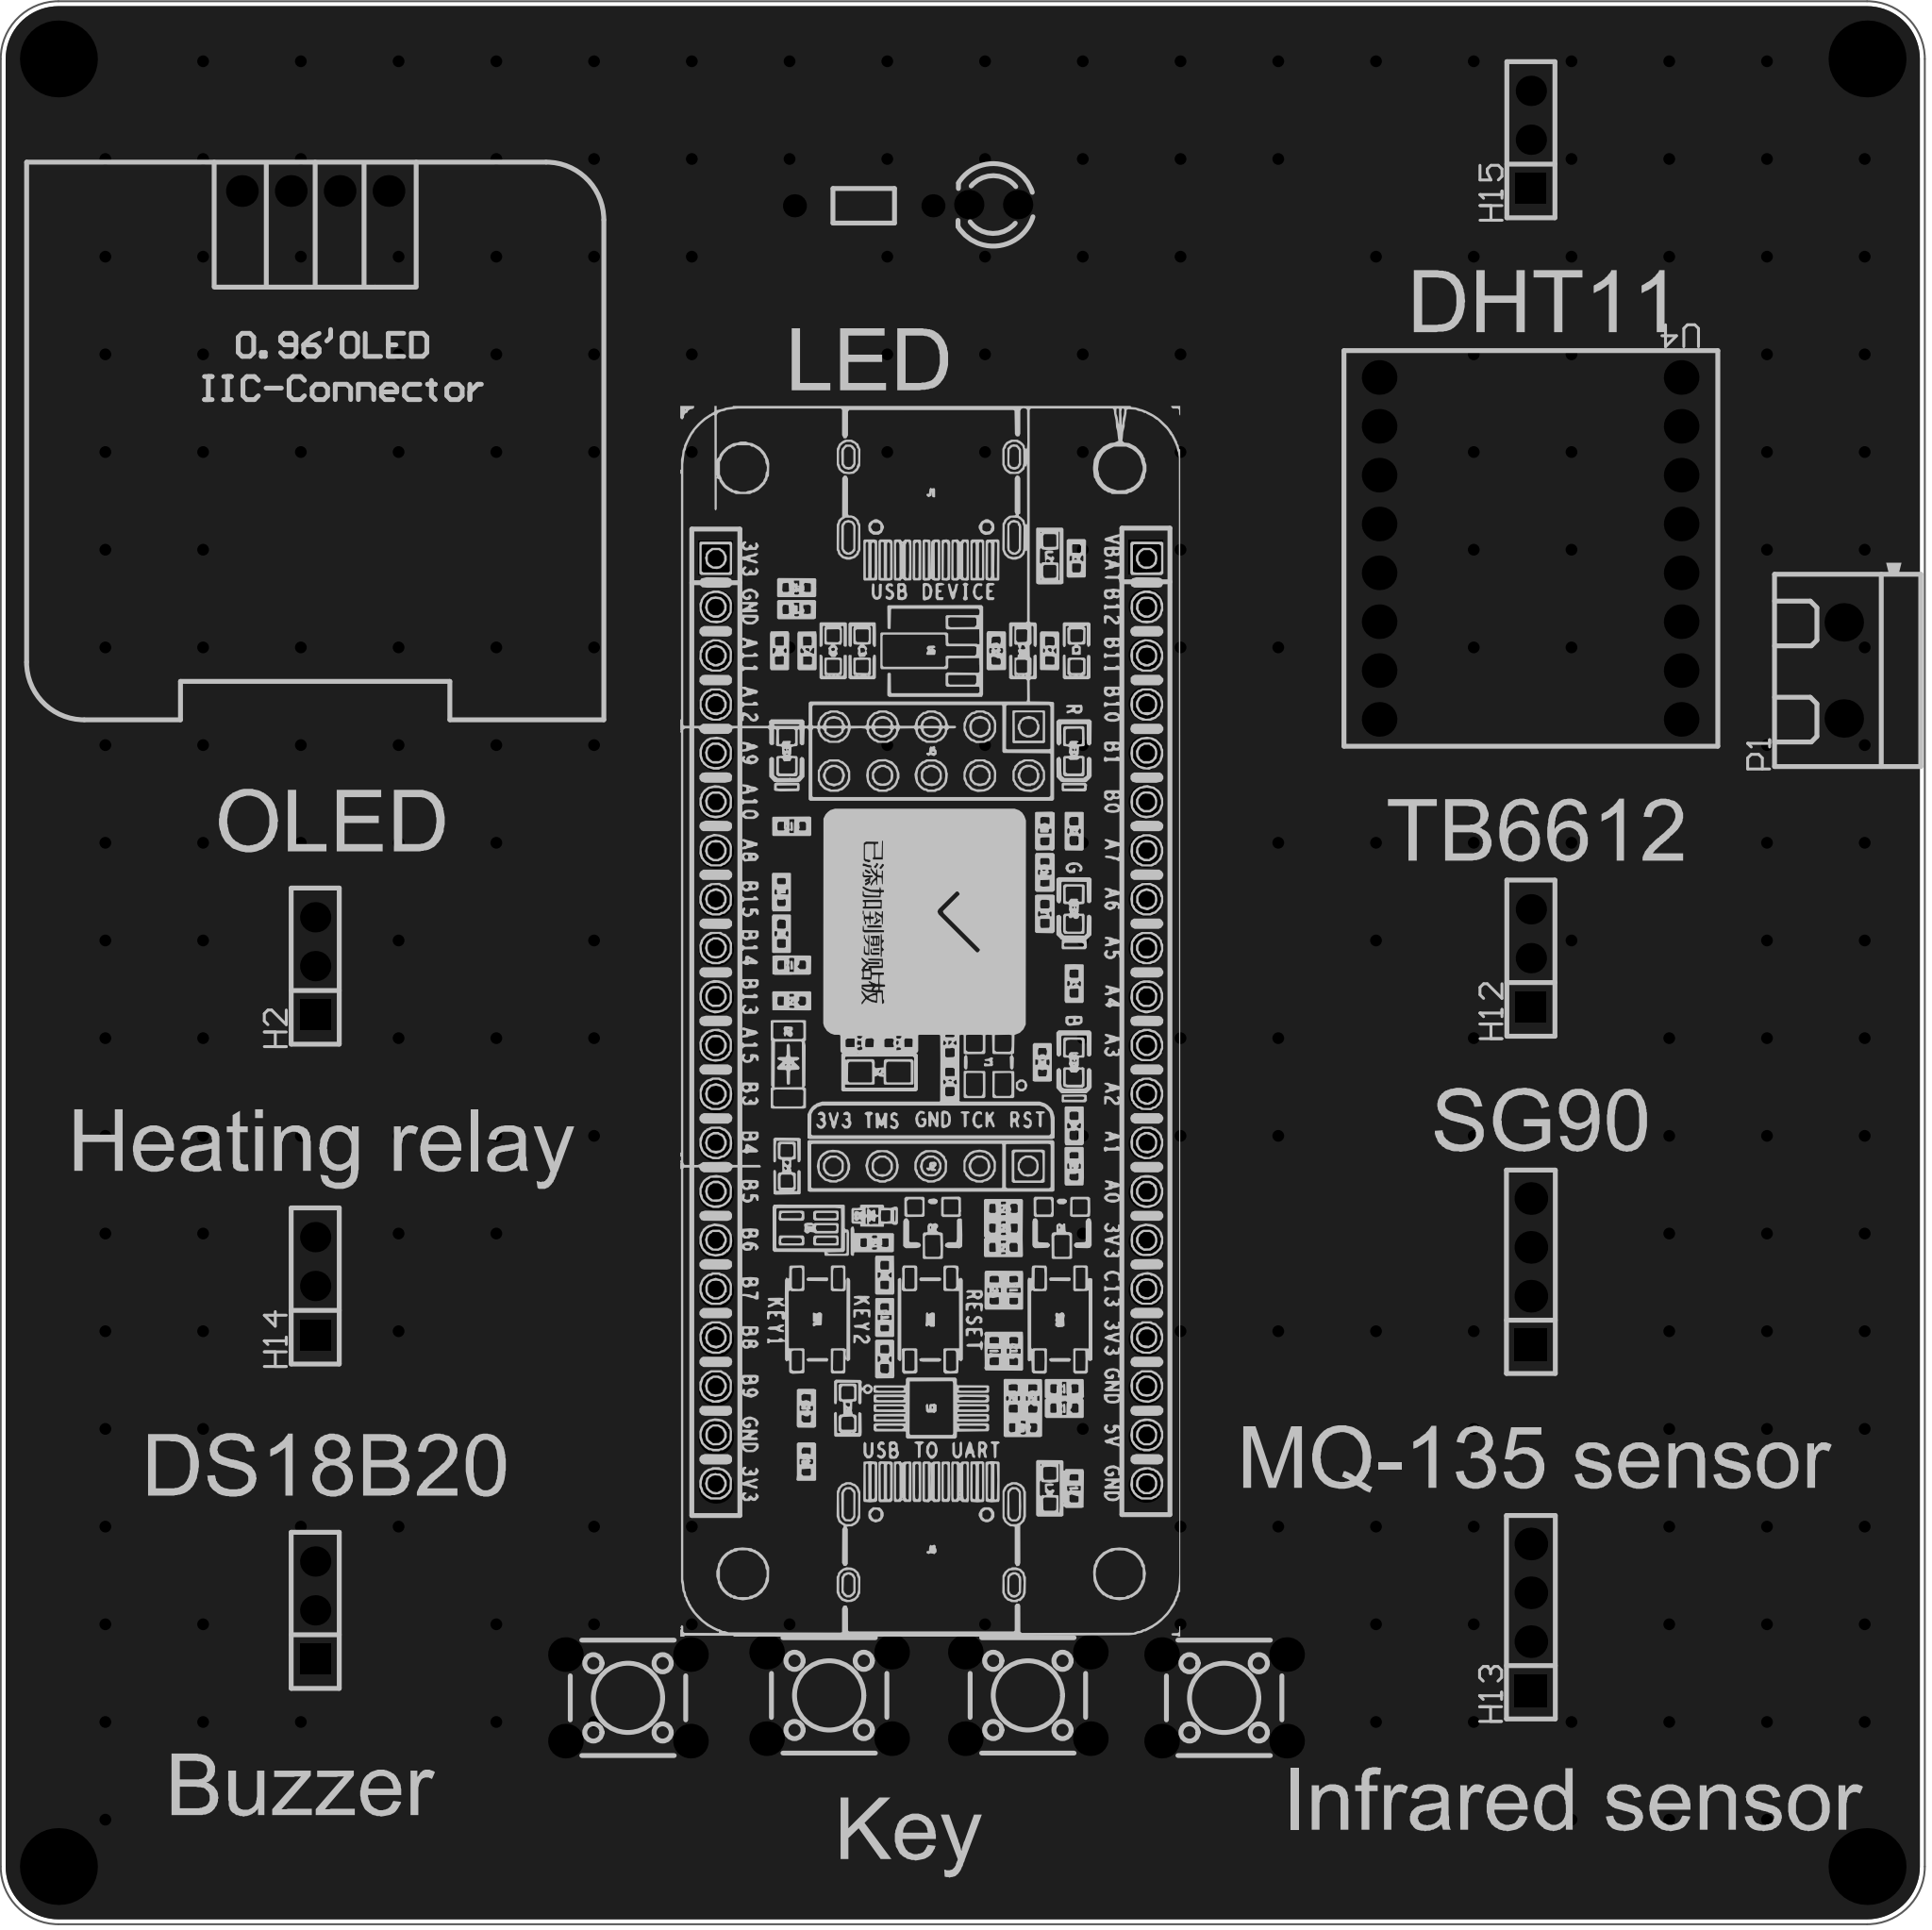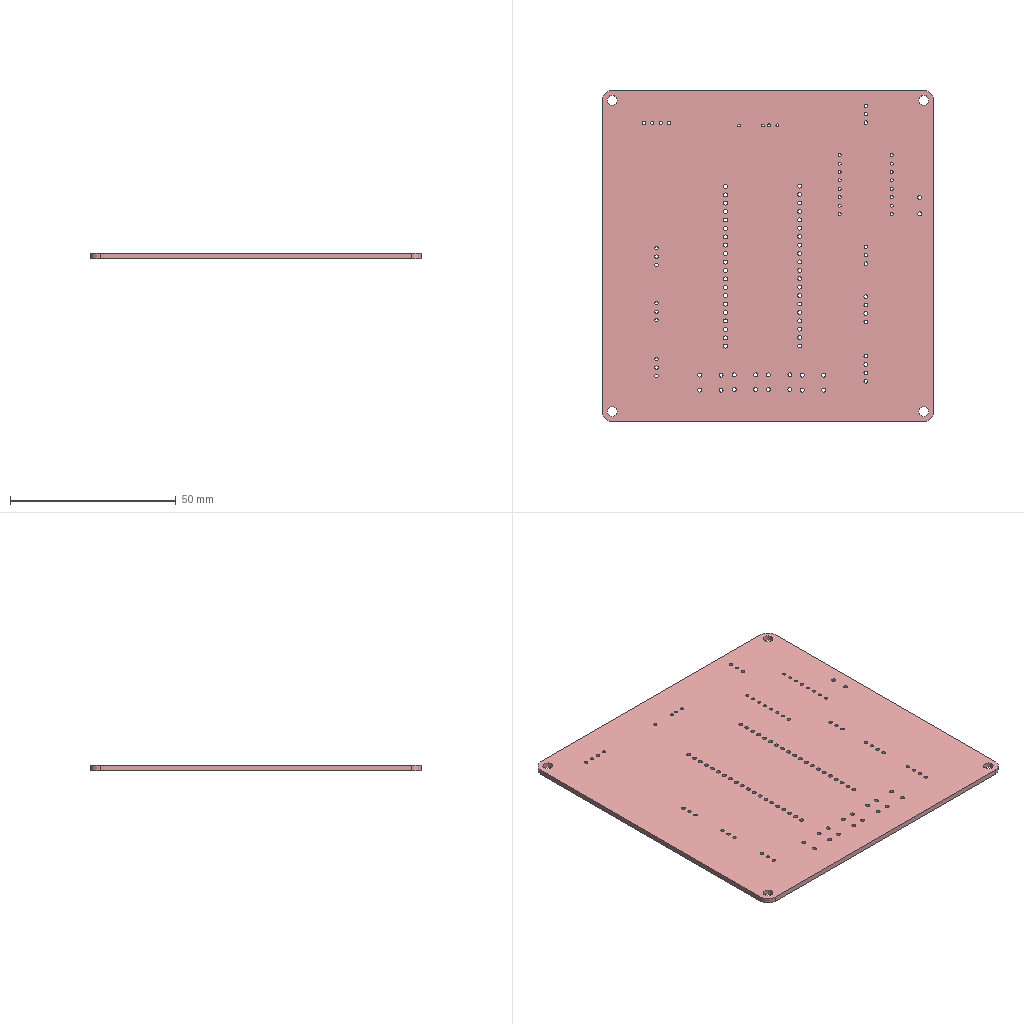Circuit board layout | Altium Designer | box 100 x 100 x 1.6 mm
Layer stack:
# Altium Designer layer stack of  (unit mm; dielectric type: 0 none, 1 core, 2 prepreg, 3 surface material)
index,name,kind,layer,copper_thickness_mm,dielectric_type,dielectric_thickness_mm,dielectric_material,dielectric_constant
0,Top Paste Mask Layer,other,,,,,,
1,Top Silkscreen Layer,other,,,,,,
2,Top Solder Mask Layer,dielectric,,,3,0.01,,3.3
3,Top Layer,copper,Top Layer,0.035,,,,
4,Dielectric1,dielectric,,,3,1.51,FR4,4.5
5,Bottom Layer,copper,Bottom Layer,0.035,,,,
6,Bottom Solder Mask Layer,dielectric,,,3,0.01,,3.3
7,Bottom Silkscreen Layer,other,,,,,,
8,Bottom Paste Mask Layer,other,,,,,,
# drill layer pairs: low layer,high layer
drill_pair,Top Layer,Bottom Layer
Part placement:
Designator,Comment,Layer,Footprint,Center-X(mm),Center-Y(mm),Rotation
SW1,,TopLayer,SW-TH_4P-L6.0-W6.0-P4.50-LS6.5,154.936,92.71,180
SW2,,TopLayer,SW-TH_4P-L6.0-W6.0-P4.50-LS6.5,134.407,92.837,180
SW3,,TopLayer,SW-TH_4P-L6.0-W6.0-P4.50-LS6.5,144.735,92.837,180
SW4,,TopLayer,SW-TH_4P-L6.0-W6.0-P4.50-LS6.5,123.952,92.71,180
H1,,TopLayer,HDR-TH_3P-P2.54-V-F,107.696,97.26,90
H4,,TopLayer,HDR-TH_4P-P2.54-V-F,170.879,114.866,90
H5,,TopLayer,HDR-TH_20P-P2.54-V-F,128.517,127.84,270
H6,,TopLayer,HDR-TH_20P-P2.54-V-F,150.869,127.888,270
LED1,,TopLayer,LED_TH-3mm,142.935,170.363,180
R1,220Ω,TopLayer,Res_1/8W,136.204,170.301,180
H2,,TopLayer,HDR-TH_3P-P2.54-V-F,107.696,130.762,90
OLED1,,TopLayer,0.96OLED_4P,107.696,171.069,0
H12,,TopLayer,HDR-TH_3P-P2.54-V-F,170.879,131.176,90
H13,,TopLayer,HDR-TH_4P-P2.54-V-F,170.879,96.902,90
H14,,TopLayer,HDR-TH_3P-P2.54-V-F,107.696,114.128,90
H15,,TopLayer,HDR-TH_3P-P2.54-V-F,170.879,173.736,90
P1,KF301-2P terminal block,TopLayer,CONN-TH_XY301V-A-5.0-2P,187.141,146.139,90
U4,,TopLayer,tb6612,170.84,152.482,180
Pad and via stacks:
# Altium Designer via and pad stacks of  (unit mm). Each distinct definition once, with the count of objects using it.
# via: kind,start_layer,end_layer,hole_mm,diameter_mm,mode(0 simple;1 top-mid-bottom;2 full stack),diameter_per_layer,count,example_net
# pad: kind,layer,hole_mm,hole_type(0 round;1 square;2 slot),plating,top_size,top_shape(1 round;2 rect;3 octagon;9 rounded rect),mid_size,bottom_size,mode,footprint,size_per_layer,count,example
pad,Multi-Layer,3,0,plated,4x4,1,4x4,4x4,0,,,4,1
pad,Multi-Layer,1.2,0,plated,1.8x1.8,1,1.8x1.8,1.8x1.8,0,SW-TH_4P-L6.0-W6.0-P4.50-LS6.5,,16,SW1.1
pad,Multi-Layer,1.02,0,plated,1.575x1.575,1,1.575x1.575,1.575x1.575,0,HDR-TH_3P-P2.54-V-F,,10,H1.3
pad,Multi-Layer,1.02,0,plated,1.575x1.575,2,1.575x1.575,1.575x1.575,0,HDR-TH_3P-P2.54-V-F,,5,H1.1
pad,Multi-Layer,1.1,0,plated,1.7x1.7,2,1.7x1.7,1.7x1.7,0,HDR-TH_4P-P2.54-V-F,,2,H4.1
pad,Multi-Layer,1.1,0,plated,1.7x1.7,1,1.7x1.7,1.7x1.7,0,HDR-TH_4P-P2.54-V-F,,6,H4.2
pad,Multi-Layer,1.2,0,plated,1.8x1.8,2,1.8x1.8,1.8x1.8,0,HDR-TH_20P-P2.54-V-F,,2,H5.1
pad,Multi-Layer,1.2,0,plated,1.8x1.8,1,1.8x1.8,1.8x1.8,0,HDR-TH_20P-P2.54-V-F,,38,H5.2
pad,Multi-Layer,0.9144,0,plated,1.524x1.524,1,1.524x1.524,1.524x1.524,0,LED_TH-3mm,,2,LED1.1
pad,Multi-Layer,0.8001,0,plated,1.199x1.199,1,1.199x1.199,1.199x1.199,0,Res_1/8W,,2,R1.1
pad,Multi-Layer,1,0,plated,1.65x1.65,1,1.65x1.65,1.65x1.65,0,0.96OLED_4P,,4,OLED1.4
pad,Multi-Layer,1.2,0,plated,2x2,1,2x2,2x2,0,CONN-TH_XY301V-A-5.0-2P,,2,P1.1
pad,Multi-Layer,0.9,0,plated,1.8x1.8,1,1.8x1.8,1.8x1.8,0,tb6612,,16,U4.1
via,Top Layer,Bottom Layer,0.3048,0.61,0,,223,GND
Copper pours:
name,layer,net,type(0 solid;1 hatched;2 none)
Bottom Layer-GND,Bottom Layer,GND,0
Top Layer-GND,Top Layer,GND,0
Design rules, without the lines most boards share:
# Altium Designer design rules of  (exported by Altium Designer, unit mm)
# columns: name | kind | enabled | priority | scope1 | scope2 | descriptor | typed fields (field=value)
Copper_copperRegion_copperThickness1oz | 0 | disabled | 4 | All | All | Clearance Constraint (Gap=5.984mil) (Disabled)(All),(All) | gap=0.152
Copper_copperRegion_copperThickness1oz_1 | 63 | disabled | 4 | All | All | Board Clearance Constraint (Gap=0mil) (Disabled)(All) |
Copper_copperRegion_Copper_copperRegion | 0 | disabled | 5 | All | All | Clearance Constraint (Gap=5.984mil) (Disabled)(All),(All) | gap=0.152
Copper_copperRegion_Copper_copperRegion_1 | 63 | disabled | 5 | All | All | Board Clearance Constraint (Gap=0mil) (Disabled)(All) |
copperThickness1oz | 0 | enabled | 6 | All | All | Clearance Constraint (Gap=5.984mil) (All),(All) | gap=0.152
copperThickness1oz_1 | 63 | enabled | 6 | All | All | Board Clearance Constraint (Gap=0mil) (All) |
copperRegion_copperThickness1oz | 20 | disabled | 1 | All | All | Polygon Connect Rule(Relief Connect )(Conductor Width=10mil) (Relief Angle=90 Angle) (Entries=4) (Air Gap Width=10mil) (Disabled)(All),(All) | connect_style(0=relief,1=direct,2=none)=0 relief_conductor_width=0.254 relief_entries=4
copperRegion_Copper_copperRegion | 20 | disabled | 2 | All | All | Polygon Connect Rule(Relief Connect )(Conductor Width=10mil) (Relief Angle=90 Angle) (Entries=4) (Air Gap Width=10mil) (Disabled)(All),(All) | connect_style(0=relief,1=direct,2=none)=0 relief_conductor_width=0.254 relief_entries=4
copperRegion | 20 | enabled | 3 | All | All | Polygon Connect Rule(Relief Connect )(Conductor Width=10mil) (Relief Angle=90 Angle) (Entries=4) (Air Gap Width=10mil) (All),(All) | connect_style(0=relief,1=direct,2=none)=0 relief_conductor_width=0.254 relief_entries=4